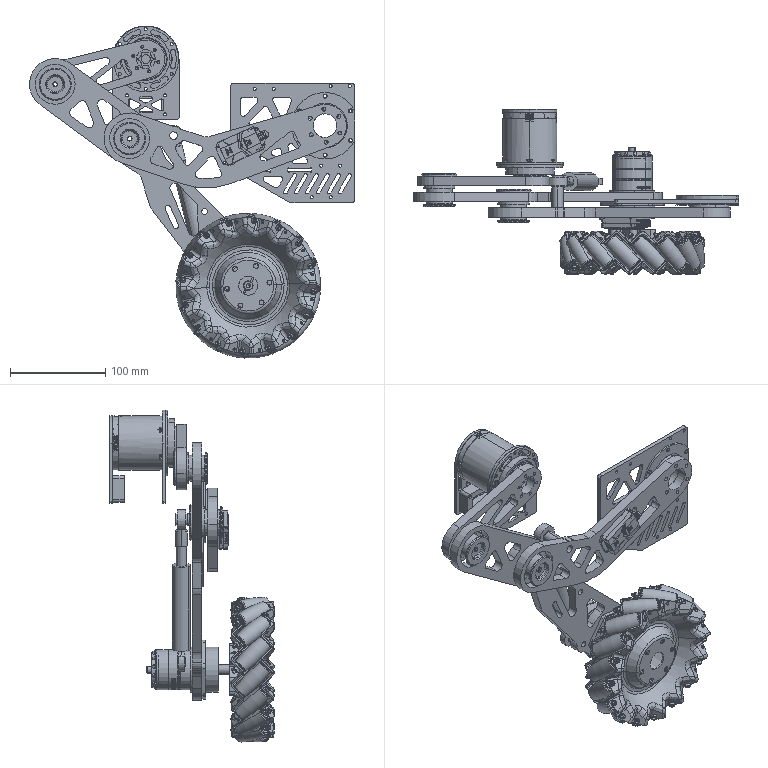Part | SolidWorks | 214 solids | 7972 faces | volume 882461 mm3 | plane 3237 | cylinder 2947 | spline 984 | cone 368 | torus 296 | sphere 140 | commonest cylinder face diameters 3.2 x212 5 x205 4 x188 10 x168 3 x140 0.2 x118